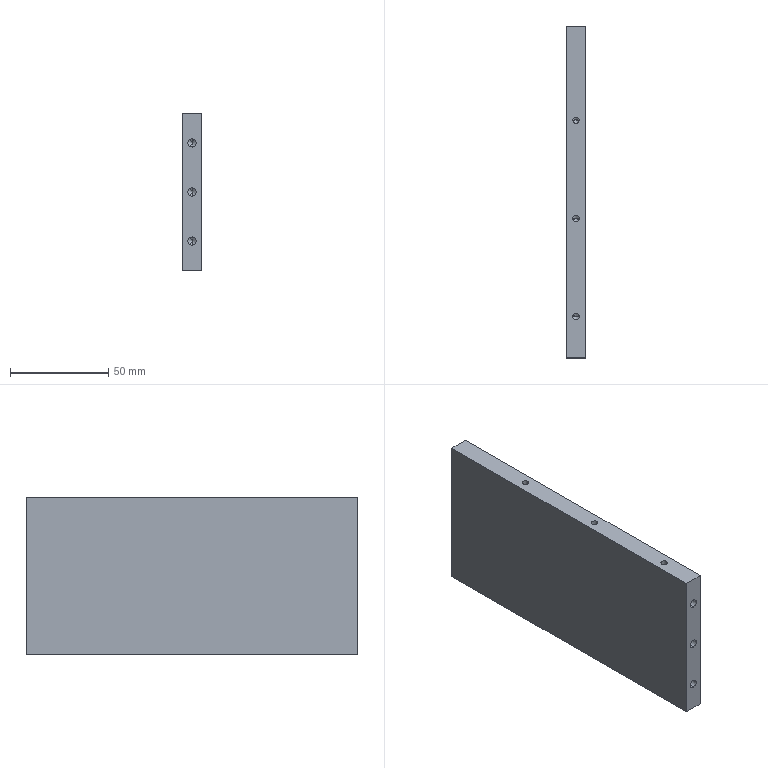Part | STEP file | 2019 Base support plate A | 1 solid | 42 faces | box 10 x 169 x 80 mm | volume 133994 mm3 | cylinder 18 | cone 18 | plane 6 | commonest cylinder face diameters 3.3 x12 4.2 x6